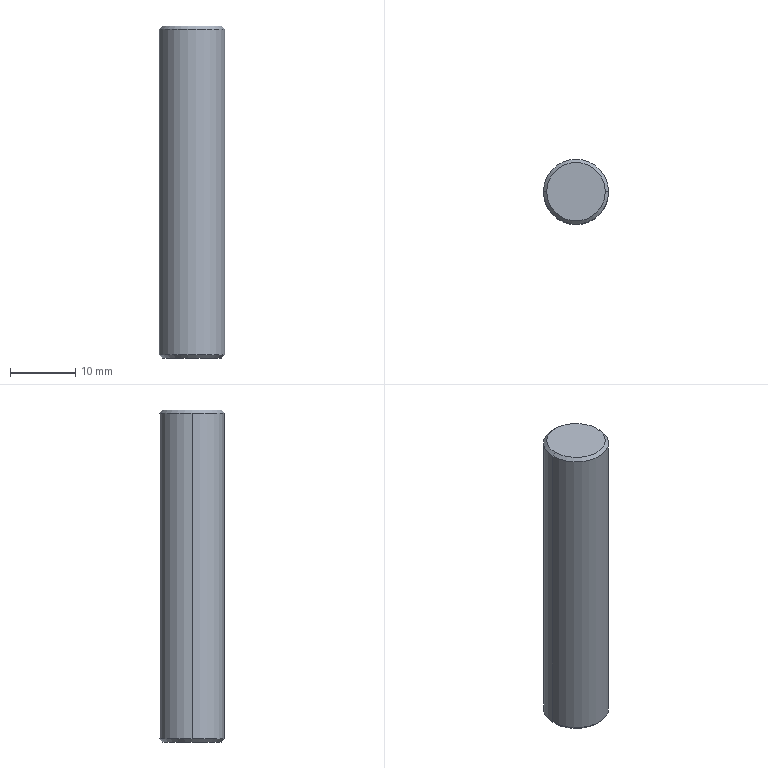Part | STEP file | (PA01.001.LX008) Tensioner Pulley Shaft | 1 solid | 8 faces | box 10 x 10 x 51 mm | volume 3998 mm3 | cone 4 | cylinder 2 | plane 2 | commonest cylinder face diameters 10 x2
STEP:
#1=CARTESIAN_POINT('',(0.,0.,0.));
#2=DIRECTION('',(0.,0.,1.));
#3=DIRECTION('',(1.,0.,0.));
#4=AXIS2_PLACEMENT_3D('',#1,#2,#3);
#5=CARTESIAN_POINT('',(-4.5,0.,-25.5));
#6=VERTEX_POINT('',#5);
#7=CARTESIAN_POINT('',(4.5,0.,-25.5));
#8=VERTEX_POINT('',#7);
#9=CARTESIAN_POINT('',(0.,0.,-25.5));
#10=DIRECTION('',(0.,0.,-1.));
#11=DIRECTION('',(1.,0.,0.));
#12=AXIS2_PLACEMENT_3D('',#9,#10,#11);
#13=CIRCLE('',#12,4.5);
#14=CARTESIAN_POINT('',(0.,0.,-25.));
#15=DIRECTION('',(0.,0.,1.));
#16=DIRECTION('',(1.,0.,0.));
#17=AXIS2_PLACEMENT_3D('',#14,#15,#16);
#18=CONICAL_SURFACE('',#17,5.,0.7854);
#19=CARTESIAN_POINT('',(6.283,-0.5));
#20=DIRECTION('',(-1.,0.));
#21=VECTOR('',#20,1.);
#22=LINE('',#19,#21);
#23=(GEOMETRIC_REPRESENTATION_CONTEXT(2)PARAMETRIC_REPRESENTATION_CONTEXT()REPRESENTATION_CONTEXT('',''));
#24=DEFINITIONAL_REPRESENTATION('',(#22),#23);
#25=PCURVE('',#18,#24);
#26=CARTESIAN_POINT('',(0.,0.,-25.5));
#27=DIRECTION('',(0.,0.,1.));
#28=DIRECTION('',(1.,0.,0.));
#29=AXIS2_PLACEMENT_3D('',#26,#27,#28);
#30=PLANE('',#29);
#31=CARTESIAN_POINT('',(4.5,0.));
#32=CARTESIAN_POINT('',(4.5,-7.794));
#33=CARTESIAN_POINT('',(-2.25,-3.897));
#34=CARTESIAN_POINT('',(-9.,0.));
#35=CARTESIAN_POINT('',(-2.25,3.897));
#36=CARTESIAN_POINT('',(4.5,7.794));
#37=CARTESIAN_POINT('',(4.5,0.));
#38=(BOUNDED_CURVE()B_SPLINE_CURVE(2,(#31,#32,#33,#34,#35,#36,#37),.UNSPECIFIED.,.T.,.F.)B_SPLINE_CURVE_WITH_KNOTS((1,2,2,2,2,1),(-2.094,0.,2.094,4.189,6.283,8.378),.UNSPECIFIED.)CURVE()GEOMETRIC_REPRESENTATION_ITEM()RATIONAL_B_SPLINE_CURVE((1.,0.5,1.,0.5,1.,0.5,1.))REPRESENTATION_ITEM(''));
#39=(GEOMETRIC_REPRESENTATION_CONTEXT(2)PARAMETRIC_REPRESENTATION_CONTEXT()REPRESENTATION_CONTEXT('',''));
#40=DEFINITIONAL_REPRESENTATION('',(#38),#39);
#41=PCURVE('',#30,#40);
#42=SURFACE_CURVE('',#13,(#25,#41),.PCURVE_S1.);
#43=EDGE_CURVE('',#6,#8,#42,.T.);
#44=ORIENTED_EDGE('',*,*,#43,.F.);
#45=CARTESIAN_POINT('',(-5.,0.,-25.));
#46=VERTEX_POINT('',#45);
#47=CARTESIAN_POINT('',(-5.,0.,-25.));
#48=DIRECTION('',(-0.7071,0.,0.7071));
#49=VECTOR('',#48,1.);
#50=LINE('',#47,#49);
#51=CARTESIAN_POINT('',(3.142,0.));
#52=DIRECTION('',(0.,1.));
#53=VECTOR('',#52,1.);
#54=LINE('',#51,#53);
#55=(GEOMETRIC_REPRESENTATION_CONTEXT(2)PARAMETRIC_REPRESENTATION_CONTEXT()REPRESENTATION_CONTEXT('',''));
#56=DEFINITIONAL_REPRESENTATION('',(#54),#55);
#57=PCURVE('',#18,#56);
#58=CARTESIAN_POINT('',(0.,0.,-25.));
#59=DIRECTION('',(0.,0.,1.));
#60=DIRECTION('',(1.,0.,0.));
#61=AXIS2_PLACEMENT_3D('',#58,#59,#60);
#62=CONICAL_SURFACE('',#61,5.,0.7854);
#63=CARTESIAN_POINT('',(3.142,0.));
#64=DIRECTION('',(0.,1.));
#65=VECTOR('',#64,1.);
#66=LINE('',#63,#65);
#67=(GEOMETRIC_REPRESENTATION_CONTEXT(2)PARAMETRIC_REPRESENTATION_CONTEXT()REPRESENTATION_CONTEXT('',''));
#68=DEFINITIONAL_REPRESENTATION('',(#66),#67);
#69=PCURVE('',#62,#68);
#70=SURFACE_CURVE('',#50,(#57,#69),.PCURVE_S1.);
#71=EDGE_CURVE('',#6,#46,#70,.T.);
#72=ORIENTED_EDGE('',*,*,#71,.T.);
#73=CARTESIAN_POINT('',(5.,0.,-25.));
#74=VERTEX_POINT('',#73);
#75=CARTESIAN_POINT('',(0.,0.,-25.));
#76=DIRECTION('',(0.,0.,1.));
#77=DIRECTION('',(1.,0.,0.));
#78=AXIS2_PLACEMENT_3D('',#75,#76,#77);
#79=CIRCLE('',#78,5.);
#80=CARTESIAN_POINT('',(0.,0.));
#81=DIRECTION('',(1.,0.));
#82=VECTOR('',#81,1.);
#83=LINE('',#80,#82);
#84=(GEOMETRIC_REPRESENTATION_CONTEXT(2)PARAMETRIC_REPRESENTATION_CONTEXT()REPRESENTATION_CONTEXT('',''));
#85=DEFINITIONAL_REPRESENTATION('',(#83),#84);
#86=PCURVE('',#18,#85);
#87=CARTESIAN_POINT('',(0.,0.,25.5));
#88=DIRECTION('',(0.,0.,-1.));
#89=DIRECTION('',(-1.,0.,0.));
#90=AXIS2_PLACEMENT_3D('',#87,#88,#89);
#91=CYLINDRICAL_SURFACE('',#90,5.);
#92=CARTESIAN_POINT('',(3.142,50.5));
#93=DIRECTION('',(-1.,0.));
#94=VECTOR('',#93,1.);
#95=LINE('',#92,#94);
#96=(GEOMETRIC_REPRESENTATION_CONTEXT(2)PARAMETRIC_REPRESENTATION_CONTEXT()REPRESENTATION_CONTEXT('',''));
#97=DEFINITIONAL_REPRESENTATION('',(#95),#96);
#98=PCURVE('',#91,#97);
#99=SURFACE_CURVE('',#79,(#86,#98),.PCURVE_S1.);
#100=EDGE_CURVE('',#74,#46,#99,.T.);
#101=ORIENTED_EDGE('',*,*,#100,.F.);
#102=CARTESIAN_POINT('',(5.,0.,-25.));
#103=DIRECTION('',(0.7071,0.,0.7071));
#104=VECTOR('',#103,1.);
#105=LINE('',#102,#104);
#106=CARTESIAN_POINT('',(0.,0.));
#107=DIRECTION('',(0.,1.));
#108=VECTOR('',#107,1.);
#109=LINE('',#106,#108);
#110=(GEOMETRIC_REPRESENTATION_CONTEXT(2)PARAMETRIC_REPRESENTATION_CONTEXT()REPRESENTATION_CONTEXT('',''));
#111=DEFINITIONAL_REPRESENTATION('',(#109),#110);
#112=PCURVE('',#18,#111);
#113=CARTESIAN_POINT('',(6.283,0.));
#114=DIRECTION('',(0.,1.));
#115=VECTOR('',#114,1.);
#116=LINE('',#113,#115);
#117=(GEOMETRIC_REPRESENTATION_CONTEXT(2)PARAMETRIC_REPRESENTATION_CONTEXT()REPRESENTATION_CONTEXT('',''));
#118=DEFINITIONAL_REPRESENTATION('',(#116),#117);
#119=PCURVE('',#62,#118);
#120=SURFACE_CURVE('',#105,(#112,#119),.PCURVE_S1.);
#121=EDGE_CURVE('',#8,#74,#120,.T.);
#122=ORIENTED_EDGE('',*,*,#121,.F.);
#123=EDGE_LOOP('',(#44,#72,#101,#122));
#124=FACE_BOUND('',#123,.T.);
#125=ADVANCED_FACE('',(#124),#18,.T.);
#126=CARTESIAN_POINT('',(4.5,0.,25.5));
#127=VERTEX_POINT('',#126);
#128=CARTESIAN_POINT('',(-4.5,0.,25.5));
#129=VERTEX_POINT('',#128);
#130=CARTESIAN_POINT('',(0.,0.,25.5));
#131=DIRECTION('',(0.,0.,1.));
#132=DIRECTION('',(1.,0.,0.));
#133=AXIS2_PLACEMENT_3D('',#130,#131,#132);
#134=CIRCLE('',#133,4.5);
#135=CARTESIAN_POINT('',(0.,0.,25.5));
#136=DIRECTION('',(0.,0.,-1.));
#137=DIRECTION('',(-1.,0.,0.));
#138=AXIS2_PLACEMENT_3D('',#135,#136,#137);
#139=CONICAL_SURFACE('',#138,4.5,0.7854);
#140=CARTESIAN_POINT('',(3.142,0.));
#141=DIRECTION('',(-1.,0.));
#142=VECTOR('',#141,1.);
#143=LINE('',#140,#142);
#144=(GEOMETRIC_REPRESENTATION_CONTEXT(2)PARAMETRIC_REPRESENTATION_CONTEXT()REPRESENTATION_CONTEXT('',''));
#145=DEFINITIONAL_REPRESENTATION('',(#143),#144);
#146=PCURVE('',#139,#145);
#147=CARTESIAN_POINT('',(0.,0.,25.5));
#148=DIRECTION('',(0.,0.,1.));
#149=DIRECTION('',(1.,0.,0.));
#150=AXIS2_PLACEMENT_3D('',#147,#148,#149);
#151=PLANE('',#150);
#152=CARTESIAN_POINT('',(0.,0.));
#153=DIRECTION('',(1.,0.));
#154=AXIS2_PLACEMENT_2D('',#152,#153);
#155=CIRCLE('',#154,4.5);
#156=(GEOMETRIC_REPRESENTATION_CONTEXT(2)PARAMETRIC_REPRESENTATION_CONTEXT()REPRESENTATION_CONTEXT('',''));
#157=DEFINITIONAL_REPRESENTATION('',(#155),#156);
#158=PCURVE('',#151,#157);
#159=SURFACE_CURVE('',#134,(#146,#158),.PCURVE_S1.);
#160=EDGE_CURVE('',#127,#129,#159,.T.);
#161=ORIENTED_EDGE('',*,*,#160,.F.);
#162=CARTESIAN_POINT('',(5.,0.,25.));
#163=VERTEX_POINT('',#162);
#164=CARTESIAN_POINT('',(4.5,0.,25.5));
#165=DIRECTION('',(0.7071,0.,-0.7071));
#166=VECTOR('',#165,1.);
#167=LINE('',#164,#166);
#168=CARTESIAN_POINT('',(3.142,0.));
#169=DIRECTION('',(0.,1.));
#170=VECTOR('',#169,1.);
#171=LINE('',#168,#170);
#172=(GEOMETRIC_REPRESENTATION_CONTEXT(2)PARAMETRIC_REPRESENTATION_CONTEXT()REPRESENTATION_CONTEXT('',''));
#173=DEFINITIONAL_REPRESENTATION('',(#171),#172);
#174=PCURVE('',#139,#173);
#175=CARTESIAN_POINT('',(0.,0.,25.5));
#176=DIRECTION('',(0.,0.,-1.));
#177=DIRECTION('',(-1.,0.,0.));
#178=AXIS2_PLACEMENT_3D('',#175,#176,#177);
#179=CONICAL_SURFACE('',#178,4.5,0.7854);
#180=CARTESIAN_POINT('',(3.142,0.));
#181=DIRECTION('',(0.,1.));
#182=VECTOR('',#181,1.);
#183=LINE('',#180,#182);
#184=(GEOMETRIC_REPRESENTATION_CONTEXT(2)PARAMETRIC_REPRESENTATION_CONTEXT()REPRESENTATION_CONTEXT('',''));
#185=DEFINITIONAL_REPRESENTATION('',(#183),#184);
#186=PCURVE('',#179,#185);
#187=SURFACE_CURVE('',#167,(#174,#186),.PCURVE_S1.);
#188=EDGE_CURVE('',#127,#163,#187,.T.);
#189=ORIENTED_EDGE('',*,*,#188,.T.);
#190=CARTESIAN_POINT('',(-5.,0.,25.));
#191=VERTEX_POINT('',#190);
#192=CARTESIAN_POINT('',(0.,0.,25.));
#193=DIRECTION('',(0.,0.,-1.));
#194=DIRECTION('',(1.,0.,0.));
#195=AXIS2_PLACEMENT_3D('',#192,#193,#194);
#196=CIRCLE('',#195,5.);
#197=CARTESIAN_POINT('',(-3.142,0.5));
#198=DIRECTION('',(1.,0.));
#199=VECTOR('',#198,1.);
#200=LINE('',#197,#199);
#201=(GEOMETRIC_REPRESENTATION_CONTEXT(2)PARAMETRIC_REPRESENTATION_CONTEXT()REPRESENTATION_CONTEXT('',''));
#202=DEFINITIONAL_REPRESENTATION('',(#200),#201);
#203=PCURVE('',#139,#202);
#204=CARTESIAN_POINT('',(-3.142,0.5));
#205=DIRECTION('',(1.,0.));
#206=VECTOR('',#205,1.);
#207=LINE('',#204,#206);
#208=(GEOMETRIC_REPRESENTATION_CONTEXT(2)PARAMETRIC_REPRESENTATION_CONTEXT()REPRESENTATION_CONTEXT('',''));
#209=DEFINITIONAL_REPRESENTATION('',(#207),#208);
#210=PCURVE('',#91,#209);
#211=SURFACE_CURVE('',#196,(#203,#210),.PCURVE_S1.);
#212=EDGE_CURVE('',#191,#163,#211,.T.);
#213=ORIENTED_EDGE('',*,*,#212,.F.);
#214=CARTESIAN_POINT('',(-4.5,0.,25.5));
#215=DIRECTION('',(-0.7071,0.,-0.7071));
#216=VECTOR('',#215,1.);
#217=LINE('',#214,#216);
#218=CARTESIAN_POINT('',(0.,0.));
#219=DIRECTION('',(0.,1.));
#220=VECTOR('',#219,1.);
#221=LINE('',#218,#220);
#222=(GEOMETRIC_REPRESENTATION_CONTEXT(2)PARAMETRIC_REPRESENTATION_CONTEXT()REPRESENTATION_CONTEXT('',''));
#223=DEFINITIONAL_REPRESENTATION('',(#221),#222);
#224=PCURVE('',#139,#223);
#225=CARTESIAN_POINT('',(6.283,0.));
#226=DIRECTION('',(0.,1.));
#227=VECTOR('',#226,1.);
#228=LINE('',#225,#227);
#229=(GEOMETRIC_REPRESENTATION_CONTEXT(2)PARAMETRIC_REPRESENTATION_CONTEXT()REPRESENTATION_CONTEXT('',''));
#230=DEFINITIONAL_REPRESENTATION('',(#228),#229);
#231=PCURVE('',#179,#230);
#232=SURFACE_CURVE('',#217,(#224,#231),.PCURVE_S1.);
#233=EDGE_CURVE('',#129,#191,#232,.T.);
#234=ORIENTED_EDGE('',*,*,#233,.F.);
#235=EDGE_LOOP('',(#161,#189,#213,#234));
#236=FACE_BOUND('',#235,.T.);
#237=ADVANCED_FACE('',(#236),#139,.T.);
#238=ORIENTED_EDGE('',*,*,#212,.T.);
#239=CARTESIAN_POINT('',(5.,0.,25.5));
#240=DIRECTION('',(0.,0.,-1.));
#241=VECTOR('',#240,1.);
#242=LINE('',#239,#241);
#243=CARTESIAN_POINT('',(3.142,0.));
#244=DIRECTION('',(0.,1.));
#245=VECTOR('',#244,1.);
#246=LINE('',#243,#245);
#247=(GEOMETRIC_REPRESENTATION_CONTEXT(2)PARAMETRIC_REPRESENTATION_CONTEXT()REPRESENTATION_CONTEXT('',''));
#248=DEFINITIONAL_REPRESENTATION('',(#246),#247);
#249=PCURVE('',#91,#248);
#250=CARTESIAN_POINT('',(0.,0.,25.5));
#251=DIRECTION('',(0.,0.,-1.));
#252=DIRECTION('',(-1.,0.,0.));
#253=AXIS2_PLACEMENT_3D('',#250,#251,#252);
#254=CYLINDRICAL_SURFACE('',#253,5.);
#255=CARTESIAN_POINT('',(3.142,0.));
#256=DIRECTION('',(0.,1.));
#257=VECTOR('',#256,1.);
#258=LINE('',#255,#257);
#259=(GEOMETRIC_REPRESENTATION_CONTEXT(2)PARAMETRIC_REPRESENTATION_CONTEXT()REPRESENTATION_CONTEXT('',''));
#260=DEFINITIONAL_REPRESENTATION('',(#258),#259);
#261=PCURVE('',#254,#260);
#262=SURFACE_CURVE('',#242,(#249,#261),.PCURVE_S1.);
#263=EDGE_CURVE('',#163,#74,#262,.T.);
#264=ORIENTED_EDGE('',*,*,#263,.T.);
#265=ORIENTED_EDGE('',*,*,#100,.T.);
#266=CARTESIAN_POINT('',(-5.,0.,25.5));
#267=DIRECTION('',(0.,0.,-1.));
#268=VECTOR('',#267,1.);
#269=LINE('',#266,#268);
#270=CARTESIAN_POINT('',(0.,0.));
#271=DIRECTION('',(0.,1.));
#272=VECTOR('',#271,1.);
#273=LINE('',#270,#272);
#274=(GEOMETRIC_REPRESENTATION_CONTEXT(2)PARAMETRIC_REPRESENTATION_CONTEXT()REPRESENTATION_CONTEXT('',''));
#275=DEFINITIONAL_REPRESENTATION('',(#273),#274);
#276=PCURVE('',#91,#275);
#277=CARTESIAN_POINT('',(6.283,0.));
#278=DIRECTION('',(0.,1.));
#279=VECTOR('',#278,1.);
#280=LINE('',#277,#279);
#281=(GEOMETRIC_REPRESENTATION_CONTEXT(2)PARAMETRIC_REPRESENTATION_CONTEXT()REPRESENTATION_CONTEXT('',''));
#282=DEFINITIONAL_REPRESENTATION('',(#280),#281);
#283=PCURVE('',#254,#282);
#284=SURFACE_CURVE('',#269,(#276,#283),.PCURVE_S1.);
#285=EDGE_CURVE('',#191,#46,#284,.T.);
#286=ORIENTED_EDGE('',*,*,#285,.F.);
#287=EDGE_LOOP('',(#238,#264,#265,#286));
#288=FACE_BOUND('',#287,.T.);
#289=ADVANCED_FACE('',(#288),#91,.T.);
#290=ORIENTED_EDGE('',*,*,#263,.F.);
#291=CARTESIAN_POINT('',(0.,0.,25.));
#292=DIRECTION('',(0.,0.,-1.));
#293=DIRECTION('',(1.,0.,0.));
#294=AXIS2_PLACEMENT_3D('',#291,#292,#293);
#295=CIRCLE('',#294,5.);
#296=CARTESIAN_POINT('',(3.142,0.5));
#297=DIRECTION('',(1.,0.));
#298=VECTOR('',#297,1.);
#299=LINE('',#296,#298);
#300=(GEOMETRIC_REPRESENTATION_CONTEXT(2)PARAMETRIC_REPRESENTATION_CONTEXT()REPRESENTATION_CONTEXT('',''));
#301=DEFINITIONAL_REPRESENTATION('',(#299),#300);
#302=PCURVE('',#254,#301);
#303=CARTESIAN_POINT('',(3.142,0.5));
#304=DIRECTION('',(1.,0.));
#305=VECTOR('',#304,1.);
#306=LINE('',#303,#305);
#307=(GEOMETRIC_REPRESENTATION_CONTEXT(2)PARAMETRIC_REPRESENTATION_CONTEXT()REPRESENTATION_CONTEXT('',''));
#308=DEFINITIONAL_REPRESENTATION('',(#306),#307);
#309=PCURVE('',#179,#308);
#310=SURFACE_CURVE('',#295,(#302,#309),.PCURVE_S1.);
#311=EDGE_CURVE('',#163,#191,#310,.T.);
#312=ORIENTED_EDGE('',*,*,#311,.T.);
#313=ORIENTED_EDGE('',*,*,#285,.T.);
#314=CARTESIAN_POINT('',(0.,0.,-25.));
#315=DIRECTION('',(0.,0.,1.));
#316=DIRECTION('',(1.,0.,0.));
#317=AXIS2_PLACEMENT_3D('',#314,#315,#316);
#318=CIRCLE('',#317,5.);
#319=CARTESIAN_POINT('',(9.425,50.5));
#320=DIRECTION('',(-1.,0.));
#321=VECTOR('',#320,1.);
#322=LINE('',#319,#321);
#323=(GEOMETRIC_REPRESENTATION_CONTEXT(2)PARAMETRIC_REPRESENTATION_CONTEXT()REPRESENTATION_CONTEXT('',''));
#324=DEFINITIONAL_REPRESENTATION('',(#322),#323);
#325=PCURVE('',#254,#324);
#326=CARTESIAN_POINT('',(0.,0.));
#327=DIRECTION('',(1.,0.));
#328=VECTOR('',#327,1.);
#329=LINE('',#326,#328);
#330=(GEOMETRIC_REPRESENTATION_CONTEXT(2)PARAMETRIC_REPRESENTATION_CONTEXT()REPRESENTATION_CONTEXT('',''));
#331=DEFINITIONAL_REPRESENTATION('',(#329),#330);
#332=PCURVE('',#62,#331);
#333=SURFACE_CURVE('',#318,(#325,#332),.PCURVE_S1.);
#334=EDGE_CURVE('',#46,#74,#333,.T.);
#335=ORIENTED_EDGE('',*,*,#334,.T.);
#336=EDGE_LOOP('',(#290,#312,#313,#335));
#337=FACE_BOUND('',#336,.T.);
#338=ADVANCED_FACE('',(#337),#254,.T.);
#339=CARTESIAN_POINT('',(0.,0.,25.5));
#340=DIRECTION('',(0.,0.,1.));
#341=DIRECTION('',(1.,0.,0.));
#342=AXIS2_PLACEMENT_3D('',#339,#340,#341);
#343=CIRCLE('',#342,4.5);
#344=CARTESIAN_POINT('',(0.,0.));
#345=DIRECTION('',(1.,0.));
#346=AXIS2_PLACEMENT_2D('',#344,#345);
#347=CIRCLE('',#346,4.5);
#348=(GEOMETRIC_REPRESENTATION_CONTEXT(2)PARAMETRIC_REPRESENTATION_CONTEXT()REPRESENTATION_CONTEXT('',''));
#349=DEFINITIONAL_REPRESENTATION('',(#347),#348);
#350=PCURVE('',#151,#349);
#351=CARTESIAN_POINT('',(9.425,0.));
#352=DIRECTION('',(-1.,0.));
#353=VECTOR('',#352,1.);
#354=LINE('',#351,#353);
#355=(GEOMETRIC_REPRESENTATION_CONTEXT(2)PARAMETRIC_REPRESENTATION_CONTEXT()REPRESENTATION_CONTEXT('',''));
#356=DEFINITIONAL_REPRESENTATION('',(#354),#355);
#357=PCURVE('',#179,#356);
#358=SURFACE_CURVE('',#343,(#350,#357),.PCURVE_S1.);
#359=EDGE_CURVE('',#129,#127,#358,.T.);
#360=ORIENTED_EDGE('',*,*,#359,.T.);
#361=ORIENTED_EDGE('',*,*,#160,.T.);
#362=EDGE_LOOP('',(#360,#361));
#363=FACE_BOUND('',#362,.T.);
#364=ADVANCED_FACE('',(#363),#151,.T.);
#365=CARTESIAN_POINT('',(0.,0.,-25.5));
#366=DIRECTION('',(0.,0.,-1.));
#367=DIRECTION('',(1.,0.,0.));
#368=AXIS2_PLACEMENT_3D('',#365,#366,#367);
#369=CIRCLE('',#368,4.5);
#370=CARTESIAN_POINT('',(4.5,0.));
#371=CARTESIAN_POINT('',(4.5,-7.794));
#372=CARTESIAN_POINT('',(-2.25,-3.897));
#373=CARTESIAN_POINT('',(-9.,0.));
#374=CARTESIAN_POINT('',(-2.25,3.897));
#375=CARTESIAN_POINT('',(4.5,7.794));
#376=CARTESIAN_POINT('',(4.5,0.));
#377=(BOUNDED_CURVE()B_SPLINE_CURVE(2,(#370,#371,#372,#373,#374,#375,#376),.UNSPECIFIED.,.T.,.F.)B_SPLINE_CURVE_WITH_KNOTS((1,2,2,2,2,1),(-2.094,0.,2.094,4.189,6.283,8.378),.UNSPECIFIED.)CURVE()GEOMETRIC_REPRESENTATION_ITEM()RATIONAL_B_SPLINE_CURVE((1.,0.5,1.,0.5,1.,0.5,1.))REPRESENTATION_ITEM(''));
#378=(GEOMETRIC_REPRESENTATION_CONTEXT(2)PARAMETRIC_REPRESENTATION_CONTEXT()REPRESENTATION_CONTEXT('',''));
#379=DEFINITIONAL_REPRESENTATION('',(#377),#378);
#380=PCURVE('',#30,#379);
#381=CARTESIAN_POINT('',(6.283,-0.5));
#382=DIRECTION('',(-1.,0.));
#383=VECTOR('',#382,1.);
#384=LINE('',#381,#383);
#385=(GEOMETRIC_REPRESENTATION_CONTEXT(2)PARAMETRIC_REPRESENTATION_CONTEXT()REPRESENTATION_CONTEXT('',''));
#386=DEFINITIONAL_REPRESENTATION('',(#384),#385);
#387=PCURVE('',#62,#386);
#388=SURFACE_CURVE('',#369,(#380,#387),.PCURVE_S1.);
#389=EDGE_CURVE('',#8,#6,#388,.T.);
#390=ORIENTED_EDGE('',*,*,#389,.T.);
#391=ORIENTED_EDGE('',*,*,#43,.T.);
#392=EDGE_LOOP('',(#390,#391));
#393=FACE_BOUND('',#392,.T.);
#394=ADVANCED_FACE('',(#393),#30,.F.);
#395=ORIENTED_EDGE('',*,*,#188,.F.);
#396=ORIENTED_EDGE('',*,*,#359,.F.);
#397=ORIENTED_EDGE('',*,*,#233,.T.);
#398=ORIENTED_EDGE('',*,*,#311,.F.);
#399=EDGE_LOOP('',(#395,#396,#397,#398));
#400=FACE_BOUND('',#399,.T.);
#401=ADVANCED_FACE('',(#400),#179,.T.);
#402=ORIENTED_EDGE('',*,*,#71,.F.);
#403=ORIENTED_EDGE('',*,*,#389,.F.);
#404=ORIENTED_EDGE('',*,*,#121,.T.);
#405=ORIENTED_EDGE('',*,*,#334,.F.);
#406=EDGE_LOOP('',(#402,#403,#404,#405));
#407=FACE_BOUND('',#406,.T.);
#408=ADVANCED_FACE('',(#407),#62,.T.);
#409=CLOSED_SHELL('',(#125,#237,#289,#338,#364,#394,#401,#408));
#410=MANIFOLD_SOLID_BREP('',#409);
#411=(LENGTH_UNIT()NAMED_UNIT(*)SI_UNIT(.MILLI.,.METRE.));
#412=UNCERTAINTY_MEASURE_WITH_UNIT(LENGTH_MEASURE(0.0000001),#411,'','');
#413=(NAMED_UNIT(*)PLANE_ANGLE_UNIT()SI_UNIT($,.RADIAN.));
#414=(NAMED_UNIT(*)SI_UNIT($,.STERADIAN.)SOLID_ANGLE_UNIT());
#415=(GEOMETRIC_REPRESENTATION_CONTEXT(3)GLOBAL_UNCERTAINTY_ASSIGNED_CONTEXT((#412))GLOBAL_UNIT_ASSIGNED_CONTEXT((#411,#413,#414))REPRESENTATION_CONTEXT('',''));
#416=ADVANCED_BREP_SHAPE_REPRESENTATION('',(#4,#410),#415);